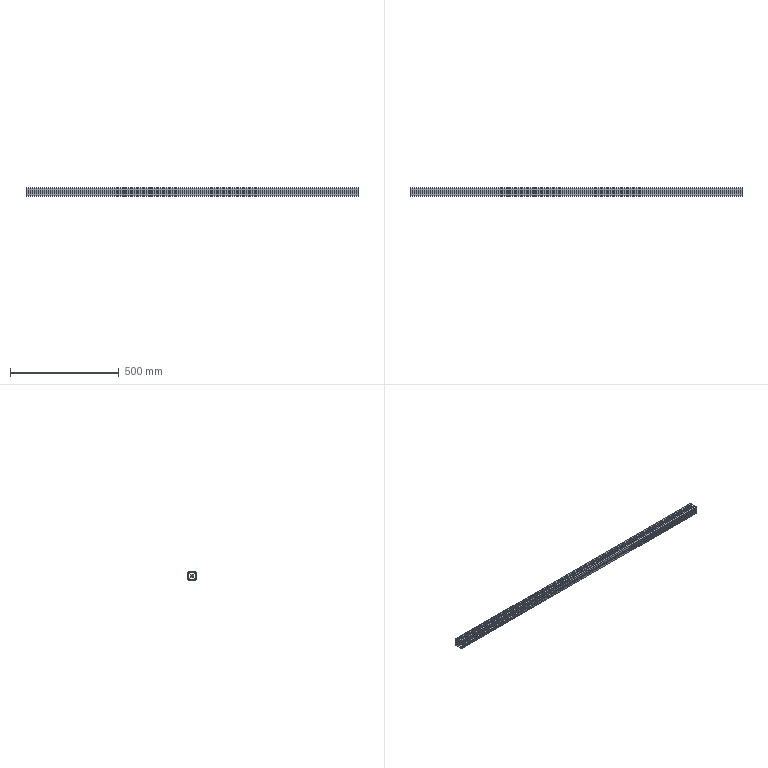Part | 1 solid | 104 faces | box 1530 x 40 x 40 mm | volume 882115 mm3 | plane 94 | cylinder 10 | commonest cylinder face diameters 5 x4 9 x4 6.8 x2